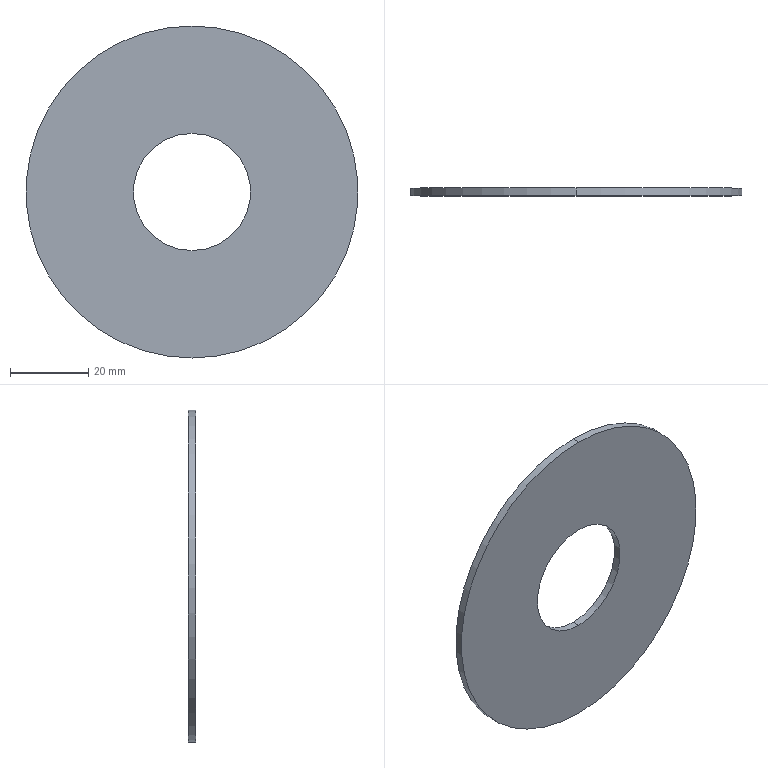Part | SolidWorks | features Extrusion 1 | 1 solid | 6 faces | box 85 x 2 x 85 mm | volume 9935 mm3 | cylinder 4 | plane 2 | commonest cylinder face diameters 30 x2 85 x2
STEP:
#1=CARTESIAN_POINT('',(0.,2.,-15.));
#2=VERTEX_POINT('',#1);
#3=CARTESIAN_POINT('',(0.,2.,15.));
#4=VERTEX_POINT('',#3);
#5=CARTESIAN_POINT('',(0.,2.,0.));
#6=DIRECTION('',(0.,1.,0.));
#7=DIRECTION('',(0.,0.,1.));
#8=AXIS2_PLACEMENT_3D('',#5,#6,#7);
#9=CIRCLE('',#8,15.);
#10=EDGE_CURVE('',#2,#4,#9,.T.);
#11=ORIENTED_EDGE('',*,*,#10,.T.);
#12=CARTESIAN_POINT('',(0.,0.,15.));
#13=VERTEX_POINT('',#12);
#14=CARTESIAN_POINT('',(0.,2.,15.));
#15=DIRECTION('',(0.,-1.,0.));
#16=VECTOR('',#15,1000.);
#17=LINE('',#14,#16);
#18=EDGE_CURVE('',#4,#13,#17,.T.);
#19=ORIENTED_EDGE('',*,*,#18,.T.);
#20=CARTESIAN_POINT('',(0.,0.,-15.));
#21=VERTEX_POINT('',#20);
#22=CARTESIAN_POINT('',(0.,0.,0.));
#23=DIRECTION('',(0.,1.,0.));
#24=DIRECTION('',(0.,0.,1.));
#25=AXIS2_PLACEMENT_3D('',#22,#23,#24);
#26=CIRCLE('',#25,15.);
#27=EDGE_CURVE('',#21,#13,#26,.T.);
#28=ORIENTED_EDGE('',*,*,#27,.F.);
#29=CARTESIAN_POINT('',(0.,2.,-15.));
#30=DIRECTION('',(0.,-1.,0.));
#31=VECTOR('',#30,1000.);
#32=LINE('',#29,#31);
#33=EDGE_CURVE('',#2,#21,#32,.T.);
#34=ORIENTED_EDGE('',*,*,#33,.F.);
#35=EDGE_LOOP('',(#11,#19,#28,#34));
#36=FACE_OUTER_BOUND('',#35,.T.);
#37=CARTESIAN_POINT('',(0.,2.,0.));
#38=DIRECTION('',(0.,-1.,0.));
#39=DIRECTION('',(0.,0.,-1.));
#40=AXIS2_PLACEMENT_3D('',#37,#38,#39);
#41=CYLINDRICAL_SURFACE('',#40,15.);
#42=ADVANCED_FACE('',(#36),#41,.F.);
#43=CARTESIAN_POINT('',(0.,2.,42.5));
#44=VERTEX_POINT('',#43);
#45=CARTESIAN_POINT('',(0.,2.,-42.5));
#46=VERTEX_POINT('',#45);
#47=CARTESIAN_POINT('',(0.,2.,0.));
#48=DIRECTION('',(0.,1.,0.));
#49=DIRECTION('',(0.,0.,1.));
#50=AXIS2_PLACEMENT_3D('',#47,#48,#49);
#51=CIRCLE('',#50,42.5);
#52=EDGE_CURVE('',#44,#46,#51,.T.);
#53=ORIENTED_EDGE('',*,*,#52,.F.);
#54=CARTESIAN_POINT('',(0.,0.,42.5));
#55=VERTEX_POINT('',#54);
#56=CARTESIAN_POINT('',(0.,2.,42.5));
#57=DIRECTION('',(0.,-1.,0.));
#58=VECTOR('',#57,1000.);
#59=LINE('',#56,#58);
#60=EDGE_CURVE('',#44,#55,#59,.T.);
#61=ORIENTED_EDGE('',*,*,#60,.T.);
#62=CARTESIAN_POINT('',(0.,0.,-42.5));
#63=VERTEX_POINT('',#62);
#64=CARTESIAN_POINT('',(0.,0.,0.));
#65=DIRECTION('',(0.,1.,0.));
#66=DIRECTION('',(0.,0.,1.));
#67=AXIS2_PLACEMENT_3D('',#64,#65,#66);
#68=CIRCLE('',#67,42.5);
#69=EDGE_CURVE('',#55,#63,#68,.T.);
#70=ORIENTED_EDGE('',*,*,#69,.T.);
#71=CARTESIAN_POINT('',(0.,2.,-42.5));
#72=DIRECTION('',(0.,-1.,0.));
#73=VECTOR('',#72,1000.);
#74=LINE('',#71,#73);
#75=EDGE_CURVE('',#46,#63,#74,.T.);
#76=ORIENTED_EDGE('',*,*,#75,.F.);
#77=EDGE_LOOP('',(#53,#61,#70,#76));
#78=FACE_OUTER_BOUND('',#77,.T.);
#79=CARTESIAN_POINT('',(0.,2.,0.));
#80=DIRECTION('',(0.,-1.,0.));
#81=DIRECTION('',(0.,0.,-1.));
#82=AXIS2_PLACEMENT_3D('',#79,#80,#81);
#83=CYLINDRICAL_SURFACE('',#82,42.5);
#84=ADVANCED_FACE('',(#78),#83,.T.);
#85=CARTESIAN_POINT('',(0.,2.,0.));
#86=DIRECTION('',(0.,1.,0.));
#87=DIRECTION('',(0.,0.,1.));
#88=AXIS2_PLACEMENT_3D('',#85,#86,#87);
#89=CIRCLE('',#88,42.5);
#90=EDGE_CURVE('',#46,#44,#89,.T.);
#91=ORIENTED_EDGE('',*,*,#90,.T.);
#92=ORIENTED_EDGE('',*,*,#52,.T.);
#93=EDGE_LOOP('',(#91,#92));
#94=FACE_OUTER_BOUND('',#93,.T.);
#95=ORIENTED_EDGE('',*,*,#10,.F.);
#96=CARTESIAN_POINT('',(0.,2.,0.));
#97=DIRECTION('',(0.,1.,0.));
#98=DIRECTION('',(0.,0.,1.));
#99=AXIS2_PLACEMENT_3D('',#96,#97,#98);
#100=CIRCLE('',#99,15.);
#101=EDGE_CURVE('',#4,#2,#100,.T.);
#102=ORIENTED_EDGE('',*,*,#101,.F.);
#103=EDGE_LOOP('',(#95,#102));
#104=FACE_BOUND('',#103,.T.);
#105=CARTESIAN_POINT('',(0.,2.,0.));
#106=DIRECTION('',(0.,1.,0.));
#107=DIRECTION('',(0.,0.,1.));
#108=AXIS2_PLACEMENT_3D('',#105,#106,#107);
#109=PLANE('',#108);
#110=ADVANCED_FACE('',(#94,#104),#109,.T.);
#111=CARTESIAN_POINT('',(0.,0.,0.));
#112=DIRECTION('',(0.,1.,0.));
#113=DIRECTION('',(0.,0.,1.));
#114=AXIS2_PLACEMENT_3D('',#111,#112,#113);
#115=CIRCLE('',#114,42.5);
#116=EDGE_CURVE('',#63,#55,#115,.T.);
#117=ORIENTED_EDGE('',*,*,#116,.F.);
#118=ORIENTED_EDGE('',*,*,#69,.F.);
#119=EDGE_LOOP('',(#117,#118));
#120=FACE_OUTER_BOUND('',#119,.T.);
#121=ORIENTED_EDGE('',*,*,#27,.T.);
#122=CARTESIAN_POINT('',(0.,0.,0.));
#123=DIRECTION('',(0.,1.,0.));
#124=DIRECTION('',(0.,0.,1.));
#125=AXIS2_PLACEMENT_3D('',#122,#123,#124);
#126=CIRCLE('',#125,15.);
#127=EDGE_CURVE('',#13,#21,#126,.T.);
#128=ORIENTED_EDGE('',*,*,#127,.T.);
#129=EDGE_LOOP('',(#121,#128));
#130=FACE_BOUND('',#129,.T.);
#131=CARTESIAN_POINT('',(0.,0.,0.));
#132=DIRECTION('',(0.,1.,0.));
#133=DIRECTION('',(0.,0.,1.));
#134=AXIS2_PLACEMENT_3D('',#131,#132,#133);
#135=PLANE('',#134);
#136=ADVANCED_FACE('',(#120,#130),#135,.F.);
#137=ORIENTED_EDGE('',*,*,#60,.F.);
#138=ORIENTED_EDGE('',*,*,#90,.F.);
#139=ORIENTED_EDGE('',*,*,#75,.T.);
#140=ORIENTED_EDGE('',*,*,#116,.T.);
#141=EDGE_LOOP('',(#137,#138,#139,#140));
#142=FACE_OUTER_BOUND('',#141,.T.);
#143=CARTESIAN_POINT('',(0.,2.,0.));
#144=DIRECTION('',(0.,-1.,0.));
#145=DIRECTION('',(0.,0.,-1.));
#146=AXIS2_PLACEMENT_3D('',#143,#144,#145);
#147=CYLINDRICAL_SURFACE('',#146,42.5);
#148=ADVANCED_FACE('',(#142),#147,.T.);
#149=ORIENTED_EDGE('',*,*,#18,.F.);
#150=ORIENTED_EDGE('',*,*,#101,.T.);
#151=ORIENTED_EDGE('',*,*,#33,.T.);
#152=ORIENTED_EDGE('',*,*,#127,.F.);
#153=EDGE_LOOP('',(#149,#150,#151,#152));
#154=FACE_OUTER_BOUND('',#153,.T.);
#155=CARTESIAN_POINT('',(0.,2.,0.));
#156=DIRECTION('',(0.,-1.,0.));
#157=DIRECTION('',(0.,0.,-1.));
#158=AXIS2_PLACEMENT_3D('',#155,#156,#157);
#159=CYLINDRICAL_SURFACE('',#158,15.);
#160=ADVANCED_FACE('',(#154),#159,.F.);
#161=CLOSED_SHELL('',(#42,#84,#110,#136,#148,#160));
#162=MANIFOLD_SOLID_BREP('',#161);
#163=CARTESIAN_POINT('',(0.,0.,0.));
#164=DIRECTION('',(0.,0.,1.));
#165=DIRECTION('',(1.,0.,0.));
#166=AXIS2_PLACEMENT_3D('',#163,#164,#165);
#167=(LENGTH_UNIT()NAMED_UNIT(*)SI_UNIT(.MILLI.,.METRE.));
#168=UNCERTAINTY_MEASURE_WITH_UNIT(LENGTH_MEASURE(0.00001),#167,'','');
#169=(NAMED_UNIT(*)PLANE_ANGLE_UNIT()SI_UNIT($,.RADIAN.));
#170=(NAMED_UNIT(*)SI_UNIT($,.STERADIAN.)SOLID_ANGLE_UNIT());
#171=(GEOMETRIC_REPRESENTATION_CONTEXT(3)GLOBAL_UNCERTAINTY_ASSIGNED_CONTEXT((#168))GLOBAL_UNIT_ASSIGNED_CONTEXT((#167,#169,#170))REPRESENTATION_CONTEXT('',''));
#172=ADVANCED_BREP_SHAPE_REPRESENTATION('',(#162,#166),#171);